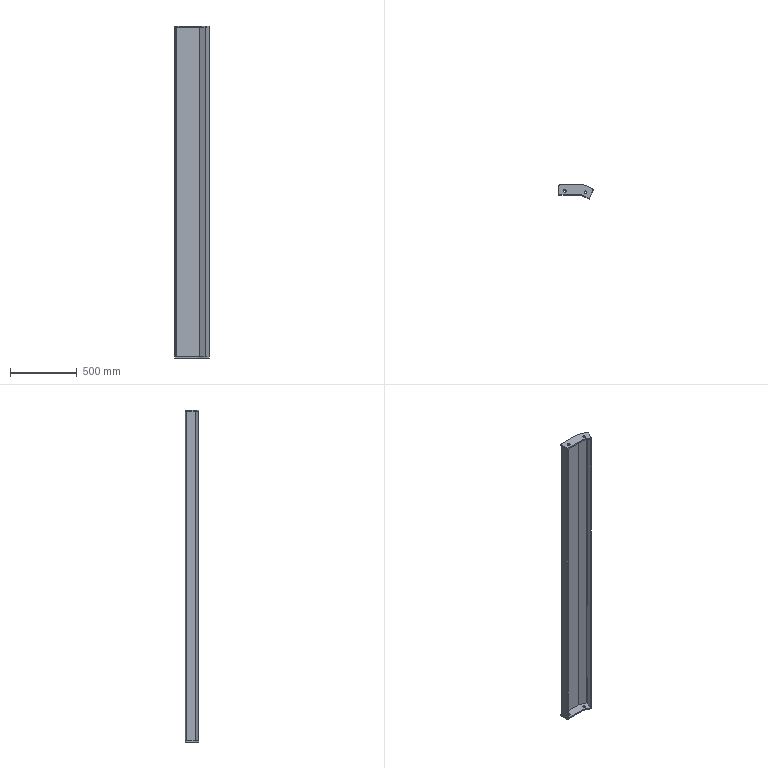Part | STEP file | Connecting beam 3_Default<As machined> | 3 solids | 60 faces | box 255.713 x 102 x 2484 mm | volume 8118407 mm3 | plane 40 | cylinder 20 | commonest cylinder face diameters 20 x9 21 x8 4 x3